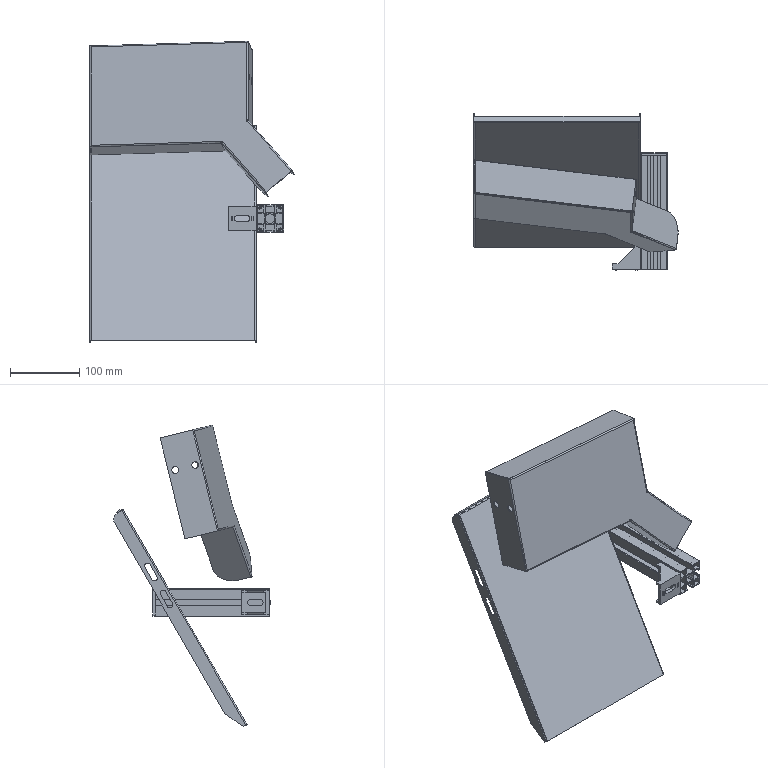Part | 5 solids | 378 faces | box 294.892 x 226.359 x 435.006 mm | volume 302021 mm3 | plane 275 | cylinder 77 | cone 24 | spline 2 | commonest cylinder face diameters 1.5 x16 1.473 x9 3.873 x9 8.4 x8 10 x8 2.2 x6